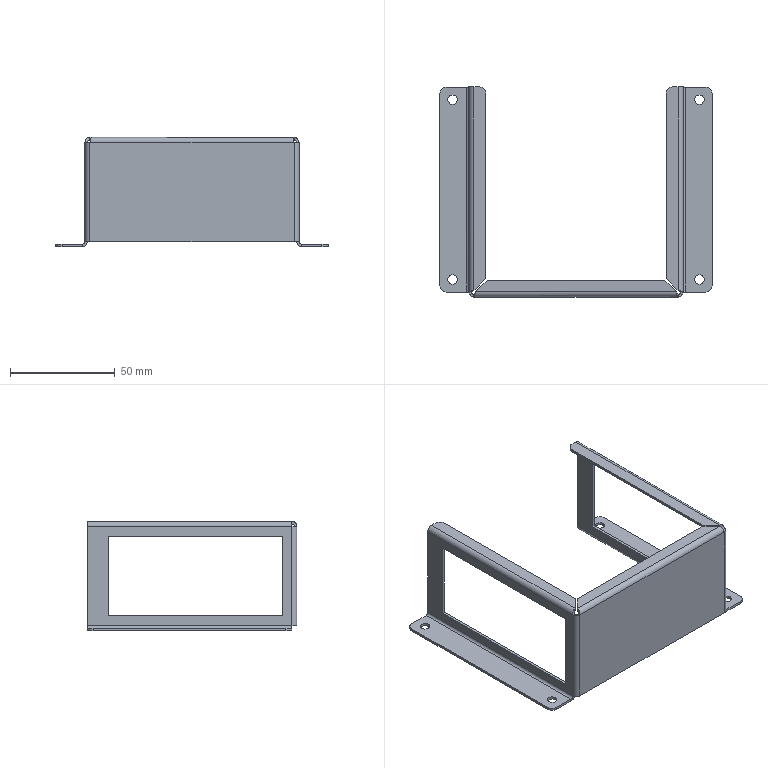Part | SolidWorks | features BaseBody 1 | 1 solid | 84 faces | box 129.6 x 100 x 52 mm | volume 15694 mm3 | plane 52 | cylinder 28 | spline 4 | commonest cylinder face diameters 4.5 x8 2.4 x7 4.8 x7 6 x6